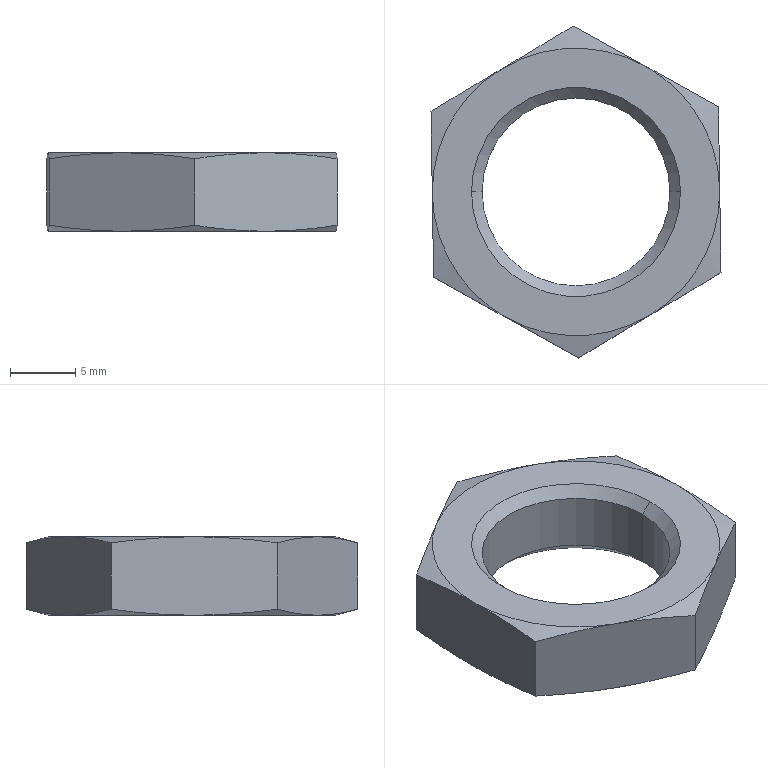Part | SolidWorks | features BaseBody 1 | 1 solid | 27 faces | box 22.195 x 25.4 x 6 mm | volume 1499 mm3 | cone 17 | plane 8 | cylinder 2 | commonest cylinder face diameters 14.376 x2
STEP:
#1=CARTESIAN_POINT('',(-187.188,0.,360.669));
#2=VERTEX_POINT('',#1);
#3=CARTESIAN_POINT('',(-172.812,0.,360.669));
#4=VERTEX_POINT('',#3);
#5=CARTESIAN_POINT('',(-180.,0.,360.669));
#6=DIRECTION('',(0.,0.,1.));
#7=DIRECTION('',(-0.8581,-0.5134,0.));
#8=AXIS2_PLACEMENT_3D('',#5,#6,#7);
#9=CIRCLE('',#8,7.188);
#10=EDGE_CURVE('',#2,#4,#9,.T.);
#11=ORIENTED_EDGE('',*,*,#10,.F.);
#12=CARTESIAN_POINT('',(-188.,0.,361.481));
#13=VERTEX_POINT('',#12);
#14=CARTESIAN_POINT('',(-188.,0.,361.481));
#15=DIRECTION('',(-0.7071,0.,0.7071));
#16=VECTOR('',#15,1000.);
#17=LINE('',#14,#16);
#18=EDGE_CURVE('',#2,#13,#17,.T.);
#19=ORIENTED_EDGE('',*,*,#18,.T.);
#20=CARTESIAN_POINT('',(-172.,0.,361.481));
#21=VERTEX_POINT('',#20);
#22=CARTESIAN_POINT('',(-180.,0.,361.481));
#23=DIRECTION('',(0.,0.,-1.));
#24=DIRECTION('',(1.,0.,0.));
#25=AXIS2_PLACEMENT_3D('',#22,#23,#24);
#26=CIRCLE('',#25,8.);
#27=EDGE_CURVE('',#21,#13,#26,.T.);
#28=ORIENTED_EDGE('',*,*,#27,.F.);
#29=CARTESIAN_POINT('',(-172.,0.,361.481));
#30=DIRECTION('',(0.7071,0.,0.7071));
#31=VECTOR('',#30,1000.);
#32=LINE('',#29,#31);
#33=EDGE_CURVE('',#4,#21,#32,.T.);
#34=ORIENTED_EDGE('',*,*,#33,.F.);
#35=EDGE_LOOP('',(#11,#19,#28,#34));
#36=FACE_OUTER_BOUND('',#35,.T.);
#37=CARTESIAN_POINT('',(-180.,0.,361.481));
#38=DIRECTION('',(0.,0.,1.));
#39=DIRECTION('',(1.,0.,0.));
#40=AXIS2_PLACEMENT_3D('',#37,#38,#39);
#41=CONICAL_SURFACE('',#40,8.,0.7854);
#42=ADVANCED_FACE('',(#36),#41,.F.);
#43=CARTESIAN_POINT('',(-187.188,0.,356.293));
#44=VERTEX_POINT('',#43);
#45=CARTESIAN_POINT('',(-180.,-7.188,356.293));
#46=VERTEX_POINT('',#45);
#47=CARTESIAN_POINT('',(-180.,0.,356.293));
#48=DIRECTION('',(0.,0.,1.));
#49=DIRECTION('',(1.,0.,0.));
#50=AXIS2_PLACEMENT_3D('',#47,#48,#49);
#51=CIRCLE('',#50,7.188);
#52=EDGE_CURVE('',#44,#46,#51,.T.);
#53=ORIENTED_EDGE('',*,*,#52,.F.);
#54=CARTESIAN_POINT('',(-187.188,0.,358.481));
#55=DIRECTION('',(0.,0.,1.));
#56=VECTOR('',#55,1000.);
#57=LINE('',#54,#56);
#58=EDGE_CURVE('',#44,#2,#57,.T.);
#59=ORIENTED_EDGE('',*,*,#58,.T.);
#60=ORIENTED_EDGE('',*,*,#10,.T.);
#61=CARTESIAN_POINT('',(-172.812,0.,356.293));
#62=VERTEX_POINT('',#61);
#63=CARTESIAN_POINT('',(-172.812,0.,358.481));
#64=DIRECTION('',(0.,0.,1.));
#65=VECTOR('',#64,1000.);
#66=LINE('',#63,#65);
#67=EDGE_CURVE('',#62,#4,#66,.T.);
#68=ORIENTED_EDGE('',*,*,#67,.F.);
#69=CARTESIAN_POINT('',(-180.,0.,356.293));
#70=DIRECTION('',(0.,0.,1.));
#71=DIRECTION('',(1.,0.,0.));
#72=AXIS2_PLACEMENT_3D('',#69,#70,#71);
#73=CIRCLE('',#72,7.188);
#74=EDGE_CURVE('',#46,#62,#73,.T.);
#75=ORIENTED_EDGE('',*,*,#74,.F.);
#76=EDGE_LOOP('',(#53,#59,#60,#68,#75));
#77=FACE_OUTER_BOUND('',#76,.T.);
#78=CARTESIAN_POINT('',(-180.,0.,358.481));
#79=DIRECTION('',(0.,0.,1.));
#80=DIRECTION('',(1.,0.,0.));
#81=AXIS2_PLACEMENT_3D('',#78,#79,#80);
#82=CYLINDRICAL_SURFACE('',#81,7.188);
#83=ADVANCED_FACE('',(#77),#82,.F.);
#84=CARTESIAN_POINT('',(-174.352,-9.44,355.481));
#85=VERTEX_POINT('',#84);
#86=CARTESIAN_POINT('',(-169.,0.,355.481));
#87=VERTEX_POINT('',#86);
#88=CARTESIAN_POINT('',(-180.,0.,355.481));
#89=DIRECTION('',(0.,0.,1.));
#90=DIRECTION('',(1.,0.,0.));
#91=AXIS2_PLACEMENT_3D('',#88,#89,#90);
#92=CIRCLE('',#91,11.);
#93=EDGE_CURVE('',#85,#87,#92,.T.);
#94=ORIENTED_EDGE('',*,*,#93,.T.);
#95=CARTESIAN_POINT('',(-168.999,0.,355.481));
#96=VERTEX_POINT('',#95);
#97=CARTESIAN_POINT('',(-167.288,0.,355.94));
#98=DIRECTION('',(0.9659,0.,0.2588));
#99=VECTOR('',#98,1000.);
#100=LINE('',#97,#99);
#101=EDGE_CURVE('',#87,#96,#100,.T.);
#102=ORIENTED_EDGE('',*,*,#101,.T.);
#103=CARTESIAN_POINT('',(-168.902,-6.179,355.937));
#104=VERTEX_POINT('',#103);
#105=CARTESIAN_POINT('',(-168.999,0.,355.481));
#106=CARTESIAN_POINT('',(-168.983,-1.035,355.486));
#107=CARTESIAN_POINT('',(-168.966,-2.067,355.53));
#108=CARTESIAN_POINT('',(-168.934,-4.126,355.687));
#109=CARTESIAN_POINT('',(-168.918,-5.153,355.8));
#110=CARTESIAN_POINT('',(-168.902,-6.179,355.937));
#111=B_SPLINE_CURVE_WITH_KNOTS('',3,(#105,#106,#107,#108,#109,#110),.UNSPECIFIED.,.F.,.F.,(4,2,4),(0.0001708,0.003269,0.006367),.UNSPECIFIED.);
#112=EDGE_CURVE('',#96,#104,#111,.T.);
#113=ORIENTED_EDGE('',*,*,#112,.T.);
#114=CARTESIAN_POINT('',(-168.902,-6.179,355.937));
#115=CARTESIAN_POINT('',(-169.807,-6.72,355.796));
#116=CARTESIAN_POINT('',(-170.713,-7.262,355.681));
#117=CARTESIAN_POINT('',(-172.529,-8.349,355.523));
#118=CARTESIAN_POINT('',(-173.439,-8.893,355.481));
#119=CARTESIAN_POINT('',(-174.352,-9.44,355.481));
#120=B_SPLINE_CURVE_WITH_KNOTS('',3,(#114,#115,#116,#117,#118,#119),.UNSPECIFIED.,.F.,.F.,(4,2,4),(0.,0.003184,0.006367),.UNSPECIFIED.);
#121=EDGE_CURVE('',#104,#85,#120,.T.);
#122=ORIENTED_EDGE('',*,*,#121,.T.);
#123=EDGE_LOOP('',(#94,#102,#113,#122));
#124=FACE_OUTER_BOUND('',#123,.T.);
#125=CARTESIAN_POINT('',(-180.,0.,355.94));
#126=DIRECTION('',(0.,0.,1.));
#127=DIRECTION('',(1.,0.,0.));
#128=AXIS2_PLACEMENT_3D('',#125,#126,#127);
#129=CONICAL_SURFACE('',#128,12.712,1.309);
#130=ADVANCED_FACE('',(#124),#129,.T.);
#131=CARTESIAN_POINT('',(-180.,7.188,356.293));
#132=VERTEX_POINT('',#131);
#133=CARTESIAN_POINT('',(-180.,0.,356.293));
#134=DIRECTION('',(0.,0.,1.));
#135=DIRECTION('',(1.,0.,0.));
#136=AXIS2_PLACEMENT_3D('',#133,#134,#135);
#137=CIRCLE('',#136,7.188);
#138=EDGE_CURVE('',#132,#44,#137,.T.);
#139=ORIENTED_EDGE('',*,*,#138,.T.);
#140=ORIENTED_EDGE('',*,*,#52,.T.);
#141=CARTESIAN_POINT('',(-180.,-8.,355.481));
#142=VERTEX_POINT('',#141);
#143=CARTESIAN_POINT('',(-180.,-8.,355.481));
#144=DIRECTION('',(0.,-0.7071,-0.7071));
#145=VECTOR('',#144,1000.);
#146=LINE('',#143,#145);
#147=EDGE_CURVE('',#46,#142,#146,.T.);
#148=ORIENTED_EDGE('',*,*,#147,.T.);
#149=CARTESIAN_POINT('',(-180.,8.,355.481));
#150=VERTEX_POINT('',#149);
#151=CARTESIAN_POINT('',(-180.,0.,355.481));
#152=DIRECTION('',(0.,0.,1.));
#153=DIRECTION('',(0.,1.,0.));
#154=AXIS2_PLACEMENT_3D('',#151,#152,#153);
#155=CIRCLE('',#154,8.);
#156=EDGE_CURVE('',#150,#142,#155,.T.);
#157=ORIENTED_EDGE('',*,*,#156,.F.);
#158=CARTESIAN_POINT('',(-180.,8.,355.481));
#159=DIRECTION('',(0.,0.7071,-0.7071));
#160=VECTOR('',#159,1000.);
#161=LINE('',#158,#160);
#162=EDGE_CURVE('',#132,#150,#161,.T.);
#163=ORIENTED_EDGE('',*,*,#162,.F.);
#164=EDGE_LOOP('',(#139,#140,#148,#157,#163));
#165=FACE_OUTER_BOUND('',#164,.T.);
#166=CARTESIAN_POINT('',(-180.,0.,355.481));
#167=DIRECTION('',(0.,0.,-1.));
#168=DIRECTION('',(0.,1.,0.));
#169=AXIS2_PLACEMENT_3D('',#166,#167,#168);
#170=CONICAL_SURFACE('',#169,8.,0.7854);
#171=ADVANCED_FACE('',(#165),#170,.F.);
#172=CARTESIAN_POINT('',(-190.999,-0.1712,361.481));
#173=VERTEX_POINT('',#172);
#174=CARTESIAN_POINT('',(-185.351,-9.611,361.481));
#175=VERTEX_POINT('',#174);
#176=CARTESIAN_POINT('',(-180.,0.,361.481));
#177=DIRECTION('',(0.,0.,1.));
#178=DIRECTION('',(-1.,0.,0.));
#179=AXIS2_PLACEMENT_3D('',#176,#177,#178);
#180=CIRCLE('',#179,11.);
#181=EDGE_CURVE('',#173,#175,#180,.T.);
#182=ORIENTED_EDGE('',*,*,#181,.T.);
#183=CARTESIAN_POINT('',(-174.352,-9.44,361.481));
#184=VERTEX_POINT('',#183);
#185=CARTESIAN_POINT('',(-180.,0.,361.481));
#186=DIRECTION('',(0.,0.,1.));
#187=DIRECTION('',(-1.,0.,0.));
#188=AXIS2_PLACEMENT_3D('',#185,#186,#187);
#189=CIRCLE('',#188,11.);
#190=EDGE_CURVE('',#175,#184,#189,.T.);
#191=ORIENTED_EDGE('',*,*,#190,.T.);
#192=CARTESIAN_POINT('',(-169.001,0.1712,361.481));
#193=VERTEX_POINT('',#192);
#194=CARTESIAN_POINT('',(-180.,0.,361.481));
#195=DIRECTION('',(0.,0.,1.));
#196=DIRECTION('',(0.,1.,0.));
#197=AXIS2_PLACEMENT_3D('',#194,#195,#196);
#198=CIRCLE('',#197,11.);
#199=EDGE_CURVE('',#184,#193,#198,.T.);
#200=ORIENTED_EDGE('',*,*,#199,.T.);
#201=CARTESIAN_POINT('',(-174.649,9.611,361.481));
#202=VERTEX_POINT('',#201);
#203=CARTESIAN_POINT('',(-180.,0.,361.481));
#204=DIRECTION('',(0.,0.,1.));
#205=DIRECTION('',(-1.,0.,0.));
#206=AXIS2_PLACEMENT_3D('',#203,#204,#205);
#207=CIRCLE('',#206,11.);
#208=EDGE_CURVE('',#193,#202,#207,.T.);
#209=ORIENTED_EDGE('',*,*,#208,.T.);
#210=CARTESIAN_POINT('',(-185.648,9.44,361.481));
#211=VERTEX_POINT('',#210);
#212=CARTESIAN_POINT('',(-180.,0.,361.481));
#213=DIRECTION('',(0.,0.,1.));
#214=DIRECTION('',(-1.,0.,0.));
#215=AXIS2_PLACEMENT_3D('',#212,#213,#214);
#216=CIRCLE('',#215,11.);
#217=EDGE_CURVE('',#202,#211,#216,.T.);
#218=ORIENTED_EDGE('',*,*,#217,.T.);
#219=CARTESIAN_POINT('',(-180.,0.,361.481));
#220=DIRECTION('',(0.,0.,1.));
#221=DIRECTION('',(0.,1.,0.));
#222=AXIS2_PLACEMENT_3D('',#219,#220,#221);
#223=CIRCLE('',#222,11.);
#224=EDGE_CURVE('',#211,#173,#223,.T.);
#225=ORIENTED_EDGE('',*,*,#224,.T.);
#226=EDGE_LOOP('',(#182,#191,#200,#209,#218,#225));
#227=FACE_OUTER_BOUND('',#226,.T.);
#228=ORIENTED_EDGE('',*,*,#27,.T.);
#229=CARTESIAN_POINT('',(-180.,0.,361.481));
#230=DIRECTION('',(0.,0.,-1.));
#231=DIRECTION('',(1.,0.,0.));
#232=AXIS2_PLACEMENT_3D('',#229,#230,#231);
#233=CIRCLE('',#232,8.);
#234=EDGE_CURVE('',#13,#21,#233,.T.);
#235=ORIENTED_EDGE('',*,*,#234,.T.);
#236=EDGE_LOOP('',(#228,#235));
#237=FACE_BOUND('',#236,.T.);
#238=CARTESIAN_POINT('',(-184.877,8.152,361.481));
#239=DIRECTION('',(0.,0.,1.));
#240=DIRECTION('',(1.,0.,0.));
#241=AXIS2_PLACEMENT_3D('',#238,#239,#240);
#242=PLANE('',#241);
#243=ADVANCED_FACE('',(#227,#237),#242,.T.);
#244=ORIENTED_EDGE('',*,*,#190,.F.);
#245=CARTESIAN_POINT('',(-179.802,-12.7,361.025));
#246=VERTEX_POINT('',#245);
#247=CARTESIAN_POINT('',(-185.351,-9.611,361.481));
#248=CARTESIAN_POINT('',(-184.421,-10.128,361.481));
#249=CARTESIAN_POINT('',(-183.495,-10.644,361.439));
#250=CARTESIAN_POINT('',(-181.645,-11.674,361.281));
#251=CARTESIAN_POINT('',(-180.723,-12.188,361.166));
#252=CARTESIAN_POINT('',(-179.802,-12.7,361.025));
#253=B_SPLINE_CURVE_WITH_KNOTS('',3,(#247,#248,#249,#250,#251,#252),.UNSPECIFIED.,.F.,.F.,(4,2,4),(0.,0.003184,0.006367),.UNSPECIFIED.);
#254=EDGE_CURVE('',#175,#246,#253,.T.);
#255=ORIENTED_EDGE('',*,*,#254,.T.);
#256=CARTESIAN_POINT('',(-179.802,-12.7,361.025));
#257=CARTESIAN_POINT('',(-178.898,-12.159,361.166));
#258=CARTESIAN_POINT('',(-177.992,-11.617,361.281));
#259=CARTESIAN_POINT('',(-176.176,-10.53,361.439));
#260=CARTESIAN_POINT('',(-175.265,-9.986,361.481));
#261=CARTESIAN_POINT('',(-174.352,-9.44,361.481));
#262=B_SPLINE_CURVE_WITH_KNOTS('',3,(#256,#257,#258,#259,#260,#261),.UNSPECIFIED.,.F.,.F.,(4,2,4),(0.,0.003184,0.006367),.UNSPECIFIED.);
#263=EDGE_CURVE('',#246,#184,#262,.T.);
#264=ORIENTED_EDGE('',*,*,#263,.T.);
#265=EDGE_LOOP('',(#244,#255,#264));
#266=FACE_OUTER_BOUND('',#265,.T.);
#267=CARTESIAN_POINT('',(-180.,0.,361.022));
#268=DIRECTION('',(0.,0.,-1.));
#269=DIRECTION('',(-1.,0.,0.));
#270=AXIS2_PLACEMENT_3D('',#267,#268,#269);
#271=CONICAL_SURFACE('',#270,12.712,1.309);
#272=ADVANCED_FACE('',(#266),#271,.T.);
#273=CARTESIAN_POINT('',(-190.9,-6.521,361.025));
#274=VERTEX_POINT('',#273);
#275=CARTESIAN_POINT('',(-190.9,-6.521,361.025));
#276=CARTESIAN_POINT('',(-189.979,-7.034,361.166));
#277=CARTESIAN_POINT('',(-189.057,-7.547,361.281));
#278=CARTESIAN_POINT('',(-187.208,-8.577,361.439));
#279=CARTESIAN_POINT('',(-186.281,-9.093,361.481));
#280=CARTESIAN_POINT('',(-185.351,-9.611,361.481));
#281=B_SPLINE_CURVE_WITH_KNOTS('',3,(#275,#276,#277,#278,#279,#280),.UNSPECIFIED.,.F.,.F.,(4,2,4),(0.,0.003184,0.006367),.UNSPECIFIED.);
#282=EDGE_CURVE('',#274,#175,#281,.T.);
#283=ORIENTED_EDGE('',*,*,#282,.T.);
#284=ORIENTED_EDGE('',*,*,#181,.F.);
#285=CARTESIAN_POINT('',(-190.999,-0.1712,361.481));
#286=CARTESIAN_POINT('',(-190.982,-1.235,361.481));
#287=CARTESIAN_POINT('',(-190.966,-2.296,361.439));
#288=CARTESIAN_POINT('',(-190.933,-4.412,361.281));
#289=CARTESIAN_POINT('',(-190.916,-5.468,361.166));
#290=CARTESIAN_POINT('',(-190.9,-6.521,361.025));
#291=B_SPLINE_CURVE_WITH_KNOTS('',3,(#285,#286,#287,#288,#289,#290),.UNSPECIFIED.,.F.,.F.,(4,2,4),(0.,0.003184,0.006367),.UNSPECIFIED.);
#292=EDGE_CURVE('',#173,#274,#291,.T.);
#293=ORIENTED_EDGE('',*,*,#292,.T.);
#294=EDGE_LOOP('',(#283,#284,#293));
#295=FACE_OUTER_BOUND('',#294,.T.);
#296=CARTESIAN_POINT('',(-180.,0.,361.022));
#297=DIRECTION('',(0.,0.,-1.));
#298=DIRECTION('',(-1.,0.,0.));
#299=AXIS2_PLACEMENT_3D('',#296,#297,#298);
#300=CONICAL_SURFACE('',#299,12.712,1.309);
#301=ADVANCED_FACE('',(#295),#300,.T.);
#302=CARTESIAN_POINT('',(-191.098,6.179,361.025));
#303=VERTEX_POINT('',#302);
#304=CARTESIAN_POINT('',(-185.648,9.44,361.481));
#305=CARTESIAN_POINT('',(-186.561,8.893,361.481));
#306=CARTESIAN_POINT('',(-187.471,8.349,361.439));
#307=CARTESIAN_POINT('',(-189.287,7.262,361.281));
#308=CARTESIAN_POINT('',(-190.193,6.72,361.166));
#309=CARTESIAN_POINT('',(-191.098,6.179,361.025));
#310=B_SPLINE_CURVE_WITH_KNOTS('',3,(#304,#305,#306,#307,#308,#309),.UNSPECIFIED.,.F.,.F.,(4,2,4),(0.,0.003184,0.006367),.UNSPECIFIED.);
#311=EDGE_CURVE('',#211,#303,#310,.T.);
#312=ORIENTED_EDGE('',*,*,#311,.T.);
#313=CARTESIAN_POINT('',(-191.098,6.179,361.025));
#314=CARTESIAN_POINT('',(-191.081,5.125,361.166));
#315=CARTESIAN_POINT('',(-191.065,4.07,361.281));
#316=CARTESIAN_POINT('',(-191.032,1.953,361.439));
#317=CARTESIAN_POINT('',(-191.015,0.8926,361.481));
#318=CARTESIAN_POINT('',(-190.999,-0.1712,361.481));
#319=B_SPLINE_CURVE_WITH_KNOTS('',3,(#313,#314,#315,#316,#317,#318),.UNSPECIFIED.,.F.,.F.,(4,2,4),(0.,0.003184,0.006367),.UNSPECIFIED.);
#320=EDGE_CURVE('',#303,#173,#319,.T.);
#321=ORIENTED_EDGE('',*,*,#320,.T.);
#322=ORIENTED_EDGE('',*,*,#224,.F.);
#323=EDGE_LOOP('',(#312,#321,#322));
#324=FACE_OUTER_BOUND('',#323,.T.);
#325=CARTESIAN_POINT('',(-180.,0.,361.022));
#326=DIRECTION('',(0.,0.,-1.));
#327=DIRECTION('',(0.,1.,0.));
#328=AXIS2_PLACEMENT_3D('',#325,#326,#327);
#329=CONICAL_SURFACE('',#328,12.712,1.309);
#330=ADVANCED_FACE('',(#324),#329,.T.);
#331=CARTESIAN_POINT('',(-180.198,12.7,361.025));
#332=VERTEX_POINT('',#331);
#333=CARTESIAN_POINT('',(-174.649,9.611,361.481));
#334=CARTESIAN_POINT('',(-175.579,10.128,361.481));
#335=CARTESIAN_POINT('',(-176.505,10.644,361.439));
#336=CARTESIAN_POINT('',(-178.355,11.674,361.281));
#337=CARTESIAN_POINT('',(-179.277,12.188,361.166));
#338=CARTESIAN_POINT('',(-180.198,12.7,361.025));
#339=B_SPLINE_CURVE_WITH_KNOTS('',3,(#333,#334,#335,#336,#337,#338),.UNSPECIFIED.,.F.,.F.,(4,2,4),(0.,0.003184,0.006367),.UNSPECIFIED.);
#340=EDGE_CURVE('',#202,#332,#339,.T.);
#341=ORIENTED_EDGE('',*,*,#340,.T.);
#342=CARTESIAN_POINT('',(-180.198,12.7,361.025));
#343=CARTESIAN_POINT('',(-181.102,12.159,361.166));
#344=CARTESIAN_POINT('',(-182.008,11.617,361.281));
#345=CARTESIAN_POINT('',(-183.824,10.53,361.439));
#346=CARTESIAN_POINT('',(-184.735,9.986,361.481));
#347=CARTESIAN_POINT('',(-185.648,9.44,361.481));
#348=B_SPLINE_CURVE_WITH_KNOTS('',3,(#342,#343,#344,#345,#346,#347),.UNSPECIFIED.,.F.,.F.,(4,2,4),(0.,0.003184,0.006367),.UNSPECIFIED.);
#349=EDGE_CURVE('',#332,#211,#348,.T.);
#350=ORIENTED_EDGE('',*,*,#349,.T.);
#351=ORIENTED_EDGE('',*,*,#217,.F.);
#352=EDGE_LOOP('',(#341,#350,#351));
#353=FACE_OUTER_BOUND('',#352,.T.);
#354=CARTESIAN_POINT('',(-180.,0.,361.022));
#355=DIRECTION('',(0.,0.,-1.));
#356=DIRECTION('',(-1.,0.,0.));
#357=AXIS2_PLACEMENT_3D('',#354,#355,#356);
#358=CONICAL_SURFACE('',#357,12.712,1.309);
#359=ADVANCED_FACE('',(#353),#358,.T.);
#360=ORIENTED_EDGE('',*,*,#208,.F.);
#361=CARTESIAN_POINT('',(-169.1,6.521,361.025));
#362=VERTEX_POINT('',#361);
#363=CARTESIAN_POINT('',(-169.001,0.1712,361.481));
#364=CARTESIAN_POINT('',(-169.018,1.235,361.481));
#365=CARTESIAN_POINT('',(-169.034,2.296,361.439));
#366=CARTESIAN_POINT('',(-169.067,4.412,361.281));
#367=CARTESIAN_POINT('',(-169.084,5.468,361.166));
#368=CARTESIAN_POINT('',(-169.1,6.521,361.025));
#369=B_SPLINE_CURVE_WITH_KNOTS('',3,(#363,#364,#365,#366,#367,#368),.UNSPECIFIED.,.F.,.F.,(4,2,4),(0.,0.003184,0.006367),.UNSPECIFIED.);
#370=EDGE_CURVE('',#193,#362,#369,.T.);
#371=ORIENTED_EDGE('',*,*,#370,.T.);
#372=CARTESIAN_POINT('',(-169.1,6.521,361.025));
#373=CARTESIAN_POINT('',(-170.021,7.034,361.166));
#374=CARTESIAN_POINT('',(-170.943,7.547,361.281));
#375=CARTESIAN_POINT('',(-172.792,8.577,361.439));
#376=CARTESIAN_POINT('',(-173.719,9.093,361.481));
#377=CARTESIAN_POINT('',(-174.649,9.611,361.481));
#378=B_SPLINE_CURVE_WITH_KNOTS('',3,(#372,#373,#374,#375,#376,#377),.UNSPECIFIED.,.F.,.F.,(4,2,4),(0.,0.003184,0.006367),.UNSPECIFIED.);
#379=EDGE_CURVE('',#362,#202,#378,.T.);
#380=ORIENTED_EDGE('',*,*,#379,.T.);
#381=EDGE_LOOP('',(#360,#371,#380));
#382=FACE_OUTER_BOUND('',#381,.T.);
#383=CARTESIAN_POINT('',(-180.,0.,361.022));
#384=DIRECTION('',(0.,0.,-1.));
#385=DIRECTION('',(-1.,0.,0.));
#386=AXIS2_PLACEMENT_3D('',#383,#384,#385);
#387=CONICAL_SURFACE('',#386,12.712,1.309);
#388=ADVANCED_FACE('',(#382),#387,.T.);
#389=ORIENTED_EDGE('',*,*,#199,.F.);
#390=CARTESIAN_POINT('',(-168.902,-6.179,361.025));
#391=VERTEX_POINT('',#390);
#392=CARTESIAN_POINT('',(-174.352,-9.44,361.481));
#393=CARTESIAN_POINT('',(-173.439,-8.893,361.481));
#394=CARTESIAN_POINT('',(-172.529,-8.349,361.439));
#395=CARTESIAN_POINT('',(-170.713,-7.262,361.281));
#396=CARTESIAN_POINT('',(-169.807,-6.72,361.166));
#397=CARTESIAN_POINT('',(-168.902,-6.179,361.025));
#398=B_SPLINE_CURVE_WITH_KNOTS('',3,(#392,#393,#394,#395,#396,#397),.UNSPECIFIED.,.F.,.F.,(4,2,4),(0.,0.003184,0.006367),.UNSPECIFIED.);
#399=EDGE_CURVE('',#184,#391,#398,.T.);
#400=ORIENTED_EDGE('',*,*,#399,.T.);
#401=CARTESIAN_POINT('',(-168.902,-6.179,361.025));
#402=CARTESIAN_POINT('',(-168.919,-5.125,361.166));
#403=CARTESIAN_POINT('',(-168.935,-4.07,361.281));
#404=CARTESIAN_POINT('',(-168.968,-1.953,361.439));
#405=CARTESIAN_POINT('',(-168.985,-0.8926,361.481));
#406=CARTESIAN_POINT('',(-169.001,0.1712,361.481));
#407=B_SPLINE_CURVE_WITH_KNOTS('',3,(#401,#402,#403,#404,#405,#406),.UNSPECIFIED.,.F.,.F.,(4,2,4),(0.,0.003184,0.006367),.UNSPECIFIED.);
#408=EDGE_CURVE('',#391,#193,#407,.T.);
#409=ORIENTED_EDGE('',*,*,#408,.T.);
#410=EDGE_LOOP('',(#389,#400,#409));
#411=FACE_OUTER_BOUND('',#410,.T.);
#412=CARTESIAN_POINT('',(-180.,0.,361.022));
#413=DIRECTION('',(0.,0.,-1.));
#414=DIRECTION('',(0.,1.,0.));
#415=AXIS2_PLACEMENT_3D('',#412,#413,#414);
#416=CONICAL_SURFACE('',#415,12.712,1.309);
#417=ADVANCED_FACE('',(#411),#416,.T.);
#418=ORIENTED_EDGE('',*,*,#18,.F.);
#419=CARTESIAN_POINT('',(-180.,0.,360.669));
#420=DIRECTION('',(0.,0.,1.));
#421=DIRECTION('',(-0.8581,-0.5134,0.));
#422=AXIS2_PLACEMENT_3D('',#419,#420,#421);
#423=CIRCLE('',#422,7.188);
#424=EDGE_CURVE('',#4,#2,#423,.T.);
#425=ORIENTED_EDGE('',*,*,#424,.F.);
#426=ORIENTED_EDGE('',*,*,#33,.T.);
#427=ORIENTED_EDGE('',*,*,#234,.F.);
#428=EDGE_LOOP('',(#418,#425,#426,#427));
#429=FACE_OUTER_BOUND('',#428,.T.);
#430=CARTESIAN_POINT('',(-180.,0.,361.481));
#431=DIRECTION('',(0.,0.,1.));
#432=DIRECTION('',(1.,0.,0.));
#433=AXIS2_PLACEMENT_3D('',#430,#431,#432);
#434=CONICAL_SURFACE('',#433,8.,0.7854);
#435=ADVANCED_FACE('',(#429),#434,.F.);
#436=CARTESIAN_POINT('',(-185.351,-9.611,355.481));
#437=VERTEX_POINT('',#436);
#438=CARTESIAN_POINT('',(-190.9,-6.521,355.937));
#439=VERTEX_POINT('',#438);
#440=CARTESIAN_POINT('',(-185.351,-9.611,355.481));
#441=CARTESIAN_POINT('',(-186.281,-9.093,355.481));
#442=CARTESIAN_POINT('',(-187.208,-8.577,355.523));
#443=CARTESIAN_POINT('',(-189.057,-7.547,355.681));
#444=CARTESIAN_POINT('',(-189.979,-7.034,355.796));
#445=CARTESIAN_POINT('',(-190.9,-6.521,355.937));
#446=B_SPLINE_CURVE_WITH_KNOTS('',3,(#440,#441,#442,#443,#444,#445),.UNSPECIFIED.,.F.,.F.,(4,2,4),(0.,0.003184,0.006367),.UNSPECIFIED.);
#447=EDGE_CURVE('',#437,#439,#446,.T.);
#448=ORIENTED_EDGE('',*,*,#447,.F.);
#449=CARTESIAN_POINT('',(-179.802,-12.7,355.937));
#450=VERTEX_POINT('',#449);
#451=CARTESIAN_POINT('',(-179.802,-12.7,355.937));
#452=CARTESIAN_POINT('',(-180.723,-12.188,355.796));
#453=CARTESIAN_POINT('',(-181.645,-11.674,355.681));
#454=CARTESIAN_POINT('',(-183.495,-10.644,355.523));
#455=CARTESIAN_POINT('',(-184.421,-10.128,355.481));
#456=CARTESIAN_POINT('',(-185.351,-9.611,355.481));
#457=B_SPLINE_CURVE_WITH_KNOTS('',3,(#451,#452,#453,#454,#455,#456),.UNSPECIFIED.,.F.,.F.,(4,2,4),(0.,0.003184,0.006367),.UNSPECIFIED.);
#458=EDGE_CURVE('',#450,#437,#457,.T.);
#459=ORIENTED_EDGE('',*,*,#458,.F.);
#460=CARTESIAN_POINT('',(-179.802,-12.7,355.481));
#461=DIRECTION('',(0.,0.,-1.));
#462=VECTOR('',#461,1000.);
#463=LINE('',#460,#462);
#464=EDGE_CURVE('',#246,#450,#463,.T.);
#465=ORIENTED_EDGE('',*,*,#464,.F.);
#466=ORIENTED_EDGE('',*,*,#254,.F.);
#467=ORIENTED_EDGE('',*,*,#282,.F.);
#468=CARTESIAN_POINT('',(-190.9,-6.521,355.481));
#469=DIRECTION('',(0.,0.,1.));
#470=VECTOR('',#469,1000.);
#471=LINE('',#468,#470);
#472=EDGE_CURVE('',#439,#274,#471,.T.);
#473=ORIENTED_EDGE('',*,*,#472,.F.);
#474=EDGE_LOOP('',(#448,#459,#465,#466,#467,#473));
#475=FACE_OUTER_BOUND('',#474,.T.);
#476=CARTESIAN_POINT('',(-190.9,-6.521,355.481));
#477=DIRECTION('',(0.4865,0.8737,0.));
#478=DIRECTION('',(-0.8737,0.4865,0.));
#479=AXIS2_PLACEMENT_3D('',#476,#477,#478);
#480=PLANE('',#479);
#481=ADVANCED_FACE('',(#475),#480,.F.);
#482=CARTESIAN_POINT('',(-174.352,-9.44,355.481));
#483=CARTESIAN_POINT('',(-175.265,-9.986,355.481));
#484=CARTESIAN_POINT('',(-176.176,-10.53,355.523));
#485=CARTESIAN_POINT('',(-177.992,-11.617,355.681));
#486=CARTESIAN_POINT('',(-178.898,-12.159,355.796));
#487=CARTESIAN_POINT('',(-179.802,-12.7,355.937));
#488=B_SPLINE_CURVE_WITH_KNOTS('',3,(#482,#483,#484,#485,#486,#487),.UNSPECIFIED.,.F.,.F.,(4,2,4),(0.,0.003184,0.006367),.UNSPECIFIED.);
#489=EDGE_CURVE('',#85,#450,#488,.T.);
#490=ORIENTED_EDGE('',*,*,#489,.F.);
#491=ORIENTED_EDGE('',*,*,#121,.F.);
#492=CARTESIAN_POINT('',(-168.902,-6.179,355.481));
#493=DIRECTION('',(0.,0.,-1.));
#494=VECTOR('',#493,1000.);
#495=LINE('',#492,#494);
#496=EDGE_CURVE('',#391,#104,#495,.T.);
#497=ORIENTED_EDGE('',*,*,#496,.F.);
#498=ORIENTED_EDGE('',*,*,#399,.F.);
#499=ORIENTED_EDGE('',*,*,#263,.F.);
#500=ORIENTED_EDGE('',*,*,#464,.T.);
#501=EDGE_LOOP('',(#490,#491,#497,#498,#499,#500));
#502=FACE_OUTER_BOUND('',#501,.T.);
#503=CARTESIAN_POINT('',(-179.802,-12.7,355.481));
#504=DIRECTION('',(-0.5134,0.8581,0.));
#505=DIRECTION('',(-0.8581,-0.5134,0.));
#506=AXIS2_PLACEMENT_3D('',#503,#504,#505);
#507=PLANE('',#506);
#508=ADVANCED_FACE('',(#502),#507,.F.);
#509=CARTESIAN_POINT('',(-191.098,6.179,355.937));
#510=VERTEX_POINT('',#509);
#511=CARTESIAN_POINT('',(-191.098,6.179,355.481));
#512=DIRECTION('',(0.,0.,1.));
#513=VECTOR('',#512,1000.);
#514=LINE('',#511,#513);
#515=EDGE_CURVE('',#510,#303,#514,.T.);
#516=ORIENTED_EDGE('',*,*,#515,.F.);
#517=CARTESIAN_POINT('',(-190.999,-0.1712,355.481));
#518=VERTEX_POINT('',#517);
#519=CARTESIAN_POINT('',(-190.999,-0.1712,355.481));
#520=CARTESIAN_POINT('',(-191.015,0.8926,355.481));
#521=CARTESIAN_POINT('',(-191.032,1.953,355.523));
#522=CARTESIAN_POINT('',(-191.065,4.07,355.681));
#523=CARTESIAN_POINT('',(-191.081,5.125,355.796));
#524=CARTESIAN_POINT('',(-191.098,6.179,355.937));
#525=B_SPLINE_CURVE_WITH_KNOTS('',3,(#519,#520,#521,#522,#523,#524),.UNSPECIFIED.,.F.,.F.,(4,2,4),(0.,0.003184,0.006367),.UNSPECIFIED.);
#526=EDGE_CURVE('',#518,#510,#525,.T.);
#527=ORIENTED_EDGE('',*,*,#526,.F.);
#528=CARTESIAN_POINT('',(-190.9,-6.521,355.937));
#529=CARTESIAN_POINT('',(-190.916,-5.468,355.796));
#530=CARTESIAN_POINT('',(-190.933,-4.412,355.681));
#531=CARTESIAN_POINT('',(-190.966,-2.296,355.523));
#532=CARTESIAN_POINT('',(-190.982,-1.235,355.481));
#533=CARTESIAN_POINT('',(-190.999,-0.1712,355.481));
#534=B_SPLINE_CURVE_WITH_KNOTS('',3,(#528,#529,#530,#531,#532,#533),.UNSPECIFIED.,.F.,.F.,(4,2,4),(0.,0.003184,0.006367),.UNSPECIFIED.);
#535=EDGE_CURVE('',#439,#518,#534,.T.);
#536=ORIENTED_EDGE('',*,*,#535,.F.);
#537=ORIENTED_EDGE('',*,*,#472,.T.);
#538=ORIENTED_EDGE('',*,*,#292,.F.);
#539=ORIENTED_EDGE('',*,*,#320,.F.);
#540=EDGE_LOOP('',(#516,#527,#536,#537,#538,#539));
#541=FACE_OUTER_BOUND('',#540,.T.);
#542=CARTESIAN_POINT('',(-191.098,6.179,355.481));
#543=DIRECTION('',(0.9999,0.01557,0.));
#544=DIRECTION('',(-0.01557,0.9999,0.));
#545=AXIS2_PLACEMENT_3D('',#542,#543,#544);
#546=PLANE('',#545);
#547=ADVANCED_FACE('',(#541),#546,.F.);
#548=CARTESIAN_POINT('',(-180.198,12.7,355.937));
#549=VERTEX_POINT('',#548);
#550=CARTESIAN_POINT('',(-180.198,12.7,355.481));
#551=DIRECTION('',(0.,0.,1.));
#552=VECTOR('',#551,1000.);
#553=LINE('',#550,#552);
#554=EDGE_CURVE('',#549,#332,#553,.T.);
#555=ORIENTED_EDGE('',*,*,#554,.F.);
#556=CARTESIAN_POINT('',(-185.648,9.44,355.481));
#557=VERTEX_POINT('',#556);
#558=CARTESIAN_POINT('',(-185.648,9.44,355.481));
#559=CARTESIAN_POINT('',(-184.735,9.986,355.481));
#560=CARTESIAN_POINT('',(-183.824,10.53,355.523));
#561=CARTESIAN_POINT('',(-182.008,11.617,355.681));
#562=CARTESIAN_POINT('',(-181.102,12.159,355.796));
#563=CARTESIAN_POINT('',(-180.198,12.7,355.937));
#564=B_SPLINE_CURVE_WITH_KNOTS('',3,(#558,#559,#560,#561,#562,#563),.UNSPECIFIED.,.F.,.F.,(4,2,4),(0.,0.003184,0.006367),.UNSPECIFIED.);
#565=EDGE_CURVE('',#557,#549,#564,.T.);
#566=ORIENTED_EDGE('',*,*,#565,.F.);
#567=CARTESIAN_POINT('',(-191.098,6.179,355.937));
#568=CARTESIAN_POINT('',(-190.193,6.72,355.796));
#569=CARTESIAN_POINT('',(-189.287,7.262,355.681));
#570=CARTESIAN_POINT('',(-187.471,8.349,355.523));
#571=CARTESIAN_POINT('',(-186.561,8.893,355.481));
#572=CARTESIAN_POINT('',(-185.648,9.44,355.481));
#573=B_SPLINE_CURVE_WITH_KNOTS('',3,(#567,#568,#569,#570,#571,#572),.UNSPECIFIED.,.F.,.F.,(4,2,4),(0.,0.003184,0.006367),.UNSPECIFIED.);
#574=EDGE_CURVE('',#510,#557,#573,.T.);
#575=ORIENTED_EDGE('',*,*,#574,.F.);
#576=ORIENTED_EDGE('',*,*,#515,.T.);
#577=ORIENTED_EDGE('',*,*,#311,.F.);
#578=ORIENTED_EDGE('',*,*,#349,.F.);
#579=EDGE_LOOP('',(#555,#566,#575,#576,#577,#578));
#580=FACE_OUTER_BOUND('',#579,.T.);
#581=CARTESIAN_POINT('',(-180.198,12.7,355.481));
#582=DIRECTION('',(0.5134,-0.8581,0.));
#583=DIRECTION('',(0.8581,0.5134,0.));
#584=AXIS2_PLACEMENT_3D('',#581,#582,#583);
#585=PLANE('',#584);
#586=ADVANCED_FACE('',(#580),#585,.F.);
#587=CARTESIAN_POINT('',(-169.1,6.521,355.937));
#588=VERTEX_POINT('',#587);
#589=CARTESIAN_POINT('',(-169.1,6.521,355.481));
#590=DIRECTION('',(0.,0.,1.));
#591=VECTOR('',#590,1000.);
#592=LINE('',#589,#591);
#593=EDGE_CURVE('',#588,#362,#592,.T.);
#594=ORIENTED_EDGE('',*,*,#593,.F.);
#595=CARTESIAN_POINT('',(-174.649,9.611,355.481));
#596=VERTEX_POINT('',#595);
#597=CARTESIAN_POINT('',(-174.649,9.611,355.481));
#598=CARTESIAN_POINT('',(-173.719,9.093,355.481));
#599=CARTESIAN_POINT('',(-172.792,8.577,355.523));
#600=CARTESIAN_POINT('',(-170.943,7.547,355.681));
#601=CARTESIAN_POINT('',(-170.021,7.034,355.796));
#602=CARTESIAN_POINT('',(-169.1,6.521,355.937));
#603=B_SPLINE_CURVE_WITH_KNOTS('',3,(#597,#598,#599,#600,#601,#602),.UNSPECIFIED.,.F.,.F.,(4,2,4),(0.,0.003184,0.006367),.UNSPECIFIED.);
#604=EDGE_CURVE('',#596,#588,#603,.T.);
#605=ORIENTED_EDGE('',*,*,#604,.F.);
#606=CARTESIAN_POINT('',(-180.198,12.7,355.937));
#607=CARTESIAN_POINT('',(-179.277,12.188,355.796));
#608=CARTESIAN_POINT('',(-178.355,11.674,355.681));
#609=CARTESIAN_POINT('',(-176.505,10.644,355.523));
#610=CARTESIAN_POINT('',(-175.579,10.128,355.481));
#611=CARTESIAN_POINT('',(-174.649,9.611,355.481));
#612=B_SPLINE_CURVE_WITH_KNOTS('',3,(#606,#607,#608,#609,#610,#611),.UNSPECIFIED.,.F.,.F.,(4,2,4),(0.,0.003184,0.006367),.UNSPECIFIED.);
#613=EDGE_CURVE('',#549,#596,#612,.T.);
#614=ORIENTED_EDGE('',*,*,#613,.F.);
#615=ORIENTED_EDGE('',*,*,#554,.T.);
#616=ORIENTED_EDGE('',*,*,#340,.F.);
#617=ORIENTED_EDGE('',*,*,#379,.F.);
#618=EDGE_LOOP('',(#594,#605,#614,#615,#616,#617));
#619=FACE_OUTER_BOUND('',#618,.T.);
#620=CARTESIAN_POINT('',(-169.1,6.521,355.481));
#621=DIRECTION('',(-0.4865,-0.8737,0.));
#622=DIRECTION('',(0.8737,-0.4865,0.));
#623=AXIS2_PLACEMENT_3D('',#620,#621,#622);
#624=PLANE('',#623);
#625=ADVANCED_FACE('',(#619),#624,.F.);
#626=CARTESIAN_POINT('',(-169.001,0.1712,355.481));
#627=VERTEX_POINT('',#626);
#628=CARTESIAN_POINT('',(-169.001,0.1712,355.481));
#629=CARTESIAN_POINT('',(-169.,0.1141,355.481));
#630=CARTESIAN_POINT('',(-169.,0.05707,355.481));
#631=CARTESIAN_POINT('',(-168.999,0.,355.481));
#632=B_SPLINE_CURVE_WITH_KNOTS('',3,(#628,#629,#630,#631),.UNSPECIFIED.,.F.,.F.,(4,4),(0.,0.0001708),.UNSPECIFIED.);
#633=EDGE_CURVE('',#627,#96,#632,.T.);
#634=ORIENTED_EDGE('',*,*,#633,.F.);
#635=CARTESIAN_POINT('',(-169.1,6.521,355.937));
#636=CARTESIAN_POINT('',(-169.084,5.468,355.796));
#637=CARTESIAN_POINT('',(-169.067,4.412,355.681));
#638=CARTESIAN_POINT('',(-169.034,2.296,355.523));
#639=CARTESIAN_POINT('',(-169.018,1.235,355.481));
#640=CARTESIAN_POINT('',(-169.001,0.1712,355.481));
#641=B_SPLINE_CURVE_WITH_KNOTS('',3,(#635,#636,#637,#638,#639,#640),.UNSPECIFIED.,.F.,.F.,(4,2,4),(0.,0.003184,0.006367),.UNSPECIFIED.);
#642=EDGE_CURVE('',#588,#627,#641,.T.);
#643=ORIENTED_EDGE('',*,*,#642,.F.);
#644=ORIENTED_EDGE('',*,*,#593,.T.);
#645=ORIENTED_EDGE('',*,*,#370,.F.);
#646=ORIENTED_EDGE('',*,*,#408,.F.);
#647=ORIENTED_EDGE('',*,*,#496,.T.);
#648=ORIENTED_EDGE('',*,*,#112,.F.);
#649=EDGE_LOOP('',(#634,#643,#644,#645,#646,#647,#648));
#650=FACE_OUTER_BOUND('',#649,.T.);
#651=CARTESIAN_POINT('',(-168.902,-6.179,355.481));
#652=DIRECTION('',(-0.9999,-0.01557,0.));
#653=DIRECTION('',(0.01557,-0.9999,0.));
#654=AXIS2_PLACEMENT_3D('',#651,#652,#653);
#655=PLANE('',#654);
#656=ADVANCED_FACE('',(#650),#655,.F.);
#657=ORIENTED_EDGE('',*,*,#58,.F.);
#658=ORIENTED_EDGE('',*,*,#138,.F.);
#659=CARTESIAN_POINT('',(-180.,0.,356.293));
#660=DIRECTION('',(0.,0.,1.));
#661=DIRECTION('',(1.,0.,0.));
#662=AXIS2_PLACEMENT_3D('',#659,#660,#661);
#663=CIRCLE('',#662,7.188);
#664=EDGE_CURVE('',#62,#132,#663,.T.);
#665=ORIENTED_EDGE('',*,*,#664,.F.);
#666=ORIENTED_EDGE('',*,*,#67,.T.);
#667=ORIENTED_EDGE('',*,*,#424,.T.);
#668=EDGE_LOOP('',(#657,#658,#665,#666,#667));
#669=FACE_OUTER_BOUND('',#668,.T.);
#670=CARTESIAN_POINT('',(-180.,0.,358.481));
#671=DIRECTION('',(0.,0.,1.));
#672=DIRECTION('',(1.,0.,0.));
#673=AXIS2_PLACEMENT_3D('',#670,#671,#672);
#674=CYLINDRICAL_SURFACE('',#673,7.188);
#675=ADVANCED_FACE('',(#669),#674,.F.);
#676=ORIENTED_EDGE('',*,*,#447,.T.);
#677=ORIENTED_EDGE('',*,*,#535,.T.);
#678=CARTESIAN_POINT('',(-180.,0.,355.481));
#679=DIRECTION('',(0.,0.,1.));
#680=DIRECTION('',(1.,0.,0.));
#681=AXIS2_PLACEMENT_3D('',#678,#679,#680);
#682=CIRCLE('',#681,11.);
#683=EDGE_CURVE('',#518,#437,#682,.T.);
#684=ORIENTED_EDGE('',*,*,#683,.T.);
#685=EDGE_LOOP('',(#676,#677,#684));
#686=FACE_OUTER_BOUND('',#685,.T.);
#687=CARTESIAN_POINT('',(-180.,0.,355.94));
#688=DIRECTION('',(0.,0.,1.));
#689=DIRECTION('',(1.,0.,0.));
#690=AXIS2_PLACEMENT_3D('',#687,#688,#689);
#691=CONICAL_SURFACE('',#690,12.712,1.309);
#692=ADVANCED_FACE('',(#686),#691,.T.);
#693=ORIENTED_EDGE('',*,*,#489,.T.);
#694=ORIENTED_EDGE('',*,*,#458,.T.);
#695=CARTESIAN_POINT('',(-180.,0.,355.481));
#696=DIRECTION('',(0.,0.,1.));
#697=DIRECTION('',(1.,0.,0.));
#698=AXIS2_PLACEMENT_3D('',#695,#696,#697);
#699=CIRCLE('',#698,11.);
#700=EDGE_CURVE('',#437,#85,#699,.T.);
#701=ORIENTED_EDGE('',*,*,#700,.T.);
#702=EDGE_LOOP('',(#693,#694,#701));
#703=FACE_OUTER_BOUND('',#702,.T.);
#704=CARTESIAN_POINT('',(-180.,0.,355.94));
#705=DIRECTION('',(0.,0.,1.));
#706=DIRECTION('',(1.,0.,0.));
#707=AXIS2_PLACEMENT_3D('',#704,#705,#706);
#708=CONICAL_SURFACE('',#707,12.712,1.309);
#709=ADVANCED_FACE('',(#703),#708,.T.);
#710=ORIENTED_EDGE('',*,*,#101,.F.);
#711=CARTESIAN_POINT('',(-180.,0.,355.481));
#712=DIRECTION('',(0.,0.,1.));
#713=DIRECTION('',(1.,0.,0.));
#714=AXIS2_PLACEMENT_3D('',#711,#712,#713);
#715=CIRCLE('',#714,11.);
#716=EDGE_CURVE('',#87,#627,#715,.T.);
#717=ORIENTED_EDGE('',*,*,#716,.T.);
#718=ORIENTED_EDGE('',*,*,#633,.T.);
#719=EDGE_LOOP('',(#710,#717,#718));
#720=FACE_OUTER_BOUND('',#719,.T.);
#721=CARTESIAN_POINT('',(-180.,0.,355.94));
#722=DIRECTION('',(0.,0.,1.));
#723=DIRECTION('',(1.,0.,0.));
#724=AXIS2_PLACEMENT_3D('',#721,#722,#723);
#725=CONICAL_SURFACE('',#724,12.712,1.309);
#726=ADVANCED_FACE('',(#720),#725,.T.);
#727=ORIENTED_EDGE('',*,*,#526,.T.);
#728=ORIENTED_EDGE('',*,*,#574,.T.);
#729=CARTESIAN_POINT('',(-180.,0.,355.481));
#730=DIRECTION('',(0.,0.,1.));
#731=DIRECTION('',(1.,0.,0.));
#732=AXIS2_PLACEMENT_3D('',#729,#730,#731);
#733=CIRCLE('',#732,11.);
#734=EDGE_CURVE('',#557,#518,#733,.T.);
#735=ORIENTED_EDGE('',*,*,#734,.T.);
#736=EDGE_LOOP('',(#727,#728,#735));
#737=FACE_OUTER_BOUND('',#736,.T.);
#738=CARTESIAN_POINT('',(-180.,0.,355.94));
#739=DIRECTION('',(0.,0.,1.));
#740=DIRECTION('',(1.,0.,0.));
#741=AXIS2_PLACEMENT_3D('',#738,#739,#740);
#742=CONICAL_SURFACE('',#741,12.712,1.309);
#743=ADVANCED_FACE('',(#737),#742,.T.);
#744=CARTESIAN_POINT('',(-180.,0.,355.481));
#745=DIRECTION('',(0.,0.,1.));
#746=DIRECTION('',(1.,0.,0.));
#747=AXIS2_PLACEMENT_3D('',#744,#745,#746);
#748=CIRCLE('',#747,11.);
#749=EDGE_CURVE('',#596,#557,#748,.T.);
#750=ORIENTED_EDGE('',*,*,#749,.T.);
#751=ORIENTED_EDGE('',*,*,#565,.T.);
#752=ORIENTED_EDGE('',*,*,#613,.T.);
#753=EDGE_LOOP('',(#750,#751,#752));
#754=FACE_OUTER_BOUND('',#753,.T.);
#755=CARTESIAN_POINT('',(-180.,0.,355.94));
#756=DIRECTION('',(0.,0.,1.));
#757=DIRECTION('',(1.,0.,0.));
#758=AXIS2_PLACEMENT_3D('',#755,#756,#757);
#759=CONICAL_SURFACE('',#758,12.712,1.309);
#760=ADVANCED_FACE('',(#754),#759,.T.);
#761=ORIENTED_EDGE('',*,*,#642,.T.);
#762=CARTESIAN_POINT('',(-180.,0.,355.481));
#763=DIRECTION('',(0.,0.,1.));
#764=DIRECTION('',(0.,-1.,0.));
#765=AXIS2_PLACEMENT_3D('',#762,#763,#764);
#766=CIRCLE('',#765,11.);
#767=EDGE_CURVE('',#627,#596,#766,.T.);
#768=ORIENTED_EDGE('',*,*,#767,.T.);
#769=ORIENTED_EDGE('',*,*,#604,.T.);
#770=EDGE_LOOP('',(#761,#768,#769));
#771=FACE_OUTER_BOUND('',#770,.T.);
#772=CARTESIAN_POINT('',(-180.,0.,355.94));
#773=DIRECTION('',(0.,0.,1.));
#774=DIRECTION('',(0.,-1.,0.));
#775=AXIS2_PLACEMENT_3D('',#772,#773,#774);
#776=CONICAL_SURFACE('',#775,12.712,1.309);
#777=ADVANCED_FACE('',(#771),#776,.T.);
#778=ORIENTED_EDGE('',*,*,#147,.F.);
#779=ORIENTED_EDGE('',*,*,#74,.T.);
#780=ORIENTED_EDGE('',*,*,#664,.T.);
#781=ORIENTED_EDGE('',*,*,#162,.T.);
#782=CARTESIAN_POINT('',(-180.,0.,355.481));
#783=DIRECTION('',(0.,0.,1.));
#784=DIRECTION('',(0.,1.,0.));
#785=AXIS2_PLACEMENT_3D('',#782,#783,#784);
#786=CIRCLE('',#785,8.);
#787=EDGE_CURVE('',#142,#150,#786,.T.);
#788=ORIENTED_EDGE('',*,*,#787,.F.);
#789=EDGE_LOOP('',(#778,#779,#780,#781,#788));
#790=FACE_OUTER_BOUND('',#789,.T.);
#791=CARTESIAN_POINT('',(-180.,0.,355.481));
#792=DIRECTION('',(0.,0.,-1.));
#793=DIRECTION('',(0.,1.,0.));
#794=AXIS2_PLACEMENT_3D('',#791,#792,#793);
#795=CONICAL_SURFACE('',#794,8.,0.7854);
#796=ADVANCED_FACE('',(#790),#795,.F.);
#797=ORIENTED_EDGE('',*,*,#156,.T.);
#798=ORIENTED_EDGE('',*,*,#787,.T.);
#799=EDGE_LOOP('',(#797,#798));
#800=FACE_BOUND('',#799,.T.);
#801=ORIENTED_EDGE('',*,*,#93,.F.);
#802=ORIENTED_EDGE('',*,*,#700,.F.);
#803=ORIENTED_EDGE('',*,*,#683,.F.);
#804=ORIENTED_EDGE('',*,*,#734,.F.);
#805=ORIENTED_EDGE('',*,*,#749,.F.);
#806=ORIENTED_EDGE('',*,*,#767,.F.);
#807=ORIENTED_EDGE('',*,*,#716,.F.);
#808=EDGE_LOOP('',(#801,#802,#803,#804,#805,#806,#807));
#809=FACE_OUTER_BOUND('',#808,.T.);
#810=CARTESIAN_POINT('',(-184.877,8.152,355.481));
#811=DIRECTION('',(0.,0.,-1.));
#812=DIRECTION('',(-1.,0.,0.));
#813=AXIS2_PLACEMENT_3D('',#810,#811,#812);
#814=PLANE('',#813);
#815=ADVANCED_FACE('',(#800,#809),#814,.T.);
#816=CLOSED_SHELL('',(#42,#83,#130,#171,#243,#272,#301,#330,#359,#388,#417,#435,#481,#508,#547,#586,#625,#656,#675,#692,#709,#726,#743,#760,#777,#796,#815));
#817=MANIFOLD_SOLID_BREP('',#816);
#818=CARTESIAN_POINT('',(0.,0.,0.));
#819=DIRECTION('',(0.,0.,1.));
#820=DIRECTION('',(1.,0.,0.));
#821=AXIS2_PLACEMENT_3D('',#818,#819,#820);
#822=(LENGTH_UNIT()NAMED_UNIT(*)SI_UNIT(.MILLI.,.METRE.));
#823=UNCERTAINTY_MEASURE_WITH_UNIT(LENGTH_MEASURE(0.00001),#822,'','');
#824=(NAMED_UNIT(*)PLANE_ANGLE_UNIT()SI_UNIT($,.RADIAN.));
#825=(NAMED_UNIT(*)SI_UNIT($,.STERADIAN.)SOLID_ANGLE_UNIT());
#826=(GEOMETRIC_REPRESENTATION_CONTEXT(3)GLOBAL_UNCERTAINTY_ASSIGNED_CONTEXT((#823))GLOBAL_UNIT_ASSIGNED_CONTEXT((#822,#824,#825))REPRESENTATION_CONTEXT('',''));
#827=ADVANCED_BREP_SHAPE_REPRESENTATION('',(#817,#821),#826);